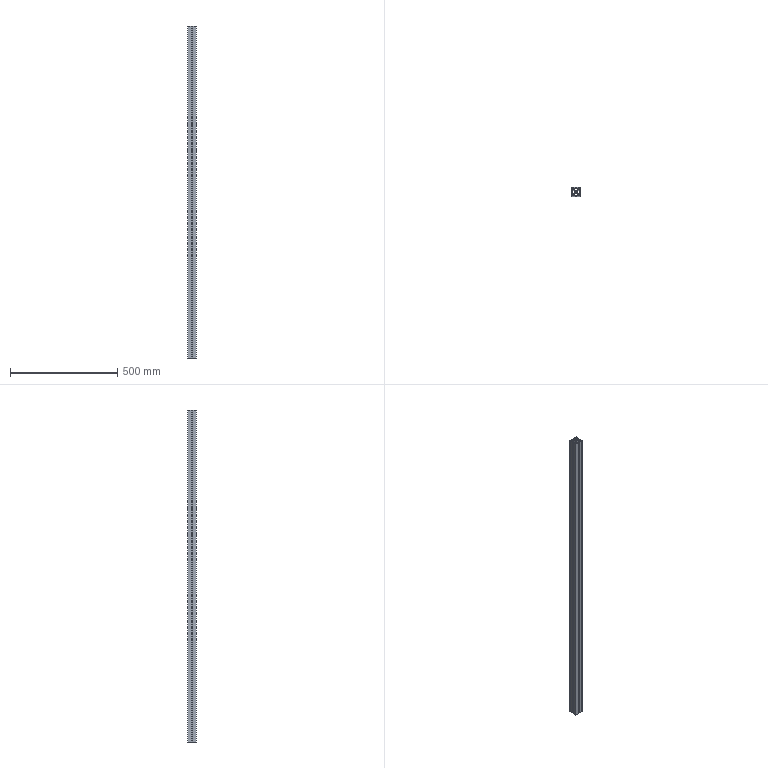Part | STEP file | ICT frame aluminum channel 1 | 1 solid | 49 faces | box 40 x 40 x 1550 mm | volume 1003296 mm3 | plane 34 | cylinder 15 | commonest cylinder face diameters 9 x8 19.803 x5 7 x2